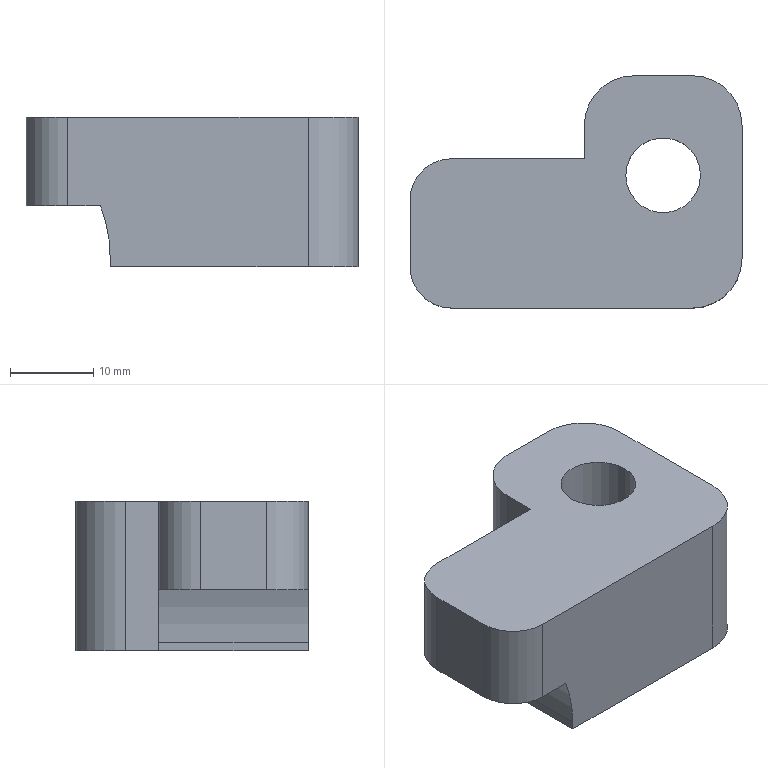Part | Creo | 1 solid | 166 faces | box 40 x 28 x 18 mm | volume 12594 mm3 | other 108 | plane 47 | cylinder 11 | commonest cylinder face diameters 12 x3 9 x2 10 x2 14 x2 1.927 x1 34.401 x1